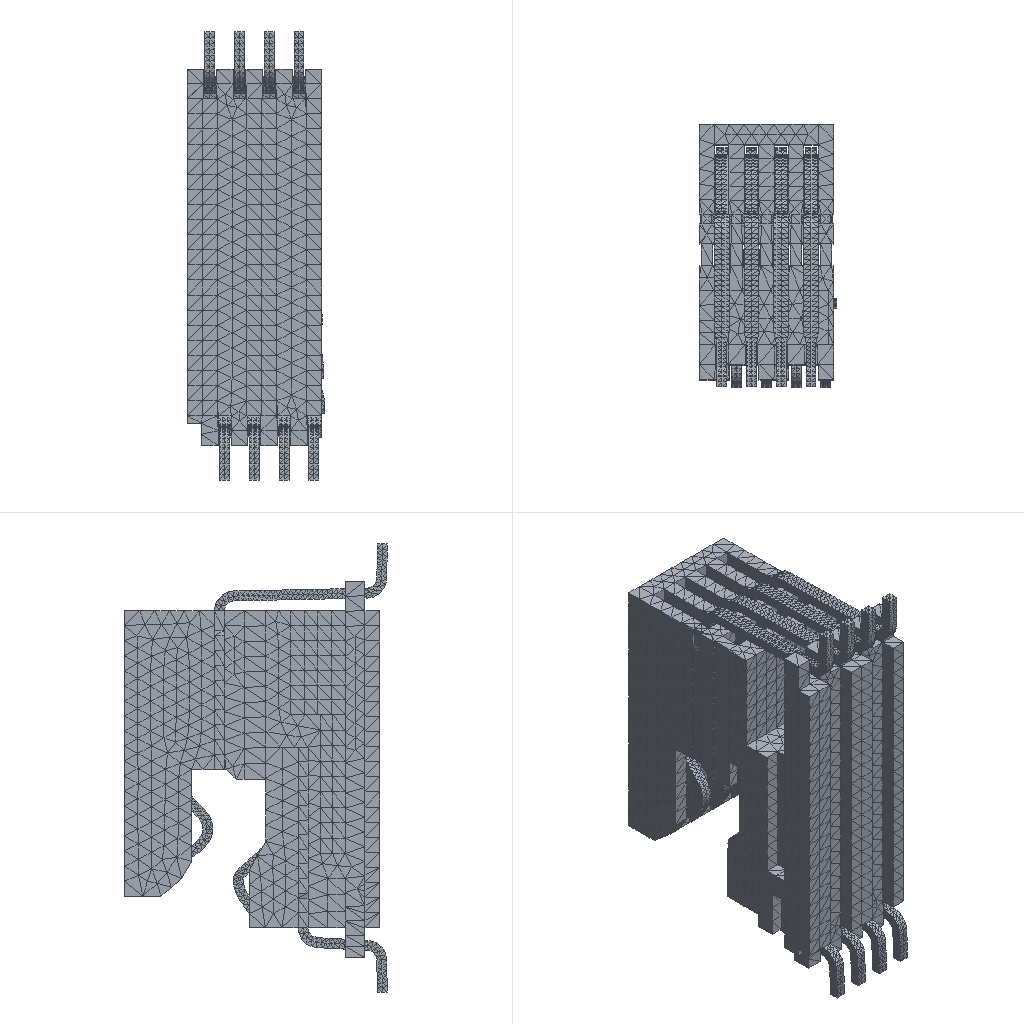Simulation study | abaqus
Set-up summary:
category,name,step,type,value,unit,region
solver,abaqus
solver,version,,,Abaqus/Standard 6.12-3
units,not stated in the deck,,not stated
analysis,deck,,coupled thermal-electrical,coupled thermal-electrical
load_step,Step-1_Temp-Ele,Step-1_Temp-Ele,coupled thermal-electrical
load_step,requested,,,1
mesh,nodes,,,107296
mesh,elements,,,59921
element_type,DC3D10E,,solid,59921
load,load commands in deck,,count,2
bc,support commands in deck,,count,2
material,C70250TM00,,in results
material,PA6T,,in results
check,setup vs results,,match,"per instance, exact: element labels, types and connectivity; labels of the nodes the elements use; coordinates of those nodes at SINGLE_PRECISION in 9 of 9 instance(s)"
Abaqus input file, long lists of numbers shortened, first 940 of 3916 lines:
*Heading
** Job name:  Model name: First_stage_TEMP-Ele
** Generated by: Abaqus/CAE 6.12-3
*Preprint, echo=NO, model=NO, history=NO, contact=NO
**
** PARTS
**
*Part, name=Housing
*Node
      1,  -9.7,  -1.59,  0.8
      2,   -7.9,  -1.59,  0.8
** (35273 more lines like these left out)
*Element, type=DC3D10E
    1,  1249,  3998,  4002,  1248,  5409,  5408,  5407,  5411,  5410,  5412
    2,  4003,  3495,   264,  1981,  5415,  5414,  5413,  5417,  5416,  5418
** (20427 more lines like these left out)
*Nset, nset=_PickedSet8, internal, generate
     1,  35275,      1
*Elset, elset=_PickedSet8, internal, generate
     1,  20429,      1
** Section: Section_PA6T
*Solid Section, elset=_PickedSet8, material=PA6T
,
*End Part
**
*Part, name=Low_T1
*Node
      1,  -7.84, -0.5128,  -1.155
      2,  -7.84,  0.2378,  -1.835
** (9275 more lines like these left out)
*Element, type=DC3D10E
   1, 1112, 1113,  412, 1114, 1521, 1520, 1519, 1523, 1522, 1524
   2, 1113, 1115, 1116, 1117, 1527, 1526, 1525, 1529, 1528, 1530
** (5131 more lines like these left out)
*Nset, nset=_PickedSet10, internal, generate
    1,  9277,     1
*Elset, elset=_PickedSet10, internal, generate
    1,  5133,     1
** Section: Section_C70250
*Solid Section, elset=_PickedSet10, material=C70250TM00
,
*End Part
**
*Part, name=Low_T2
*Node
      1,  -8.44, -0.5128,  -1.155
      2,  -8.44,  0.2378,  -1.835
** (9583 more lines like these left out)
*Element, type=DC3D10E
   1, 1123, 1124, 1125, 1126, 1561, 1560, 1559, 1563, 1562, 1564
   2, 1123, 1127, 1128, 1129, 1567, 1566, 1565, 1569, 1568, 1570
** (5348 more lines like these left out)
*Nset, nset=_PickedSet6, internal, generate
    1,  9585,     1
*Elset, elset=_PickedSet6, internal, generate
    1,  5350,     1
** Section: Section_C70250
*Solid Section, elset=_PickedSet6, material=C70250TM00
,
*End Part
**
*Part, name=Low_T3
*Node
      1,  -9.04, -0.5128,  -1.155
      2,  -9.04,  0.2378,  -1.835
** (9164 more lines like these left out)
*Element, type=DC3D10E
   1, 1113, 1114, 1115, 1116, 1509, 1508, 1507, 1511, 1510, 1512
   2, 1116, 1117,  884, 1113, 1515, 1514, 1513, 1511, 1516, 1517
** (5043 more lines like these left out)
*Nset, nset=_PickedSet8, internal, generate
    1,  9166,     1
*Elset, elset=_PickedSet8, internal, generate
    1,  5045,     1
** Section: Section_C70250
*Solid Section, elset=_PickedSet8, material=C70250TM00
,
*End Part
**
*Part, name=Low_T4
*Node
      1,  -9.64, -0.5128,  -1.155
      2,  -9.64,  0.2378,  -1.835
** (9299 more lines like these left out)
*Element, type=DC3D10E
   1, 1117, 1118, 1119, 1120, 1524, 1523, 1522, 1526, 1525, 1527
   2, 1121, 1117, 1118, 1119, 1529, 1524, 1528, 1530, 1522, 1523
** (5144 more lines like these left out)
*Nset, nset=_PickedSet6, internal, generate
    1,  9301,     1
*Elset, elset=_PickedSet6, internal, generate
    1,  5146,     1
** Section: Section_C70250
*Solid Section, elset=_PickedSet6, material=C70250TM00
,
*End Part
**
*Part, name=UP_T1
*Node
      1,  -8.15,  -2.78,   4.05
      2,  -8.15,  -2.79,         4.75
** (8647 more lines like these left out)
*Element, type=DC3D10E
   1, 1087, 1088, 1089, 1090, 1441, 1440, 1439, 1443, 1442, 1444
   2, 1087, 1091, 1092, 1093, 1447, 1446, 1445, 1449, 1448, 1450
** (4688 more lines like these left out)
*Nset, nset=_PickedSet6, internal, generate
    1,  8649,     1
*Elset, elset=_PickedSet6, internal, generate
    1,  4690,     1
** Section: Section_C70250
*Solid Section, elset=_PickedSet6, material=C70250TM00
,
*End Part
**
*Part, name=UP_T2
*Node
      1,        -8.75,  -2.78,   4.05
      2,        -8.75,  -2.79,         4.75
** (8659 more lines like these left out)
*Element, type=DC3D10E
   1, 1085, 1086, 1087,  928, 1444, 1443, 1442, 1446, 1445, 1447
   2, 1085, 1087, 1086,  893, 1442, 1443, 1444, 1449, 1448, 1450
** (4696 more lines like these left out)
*Nset, nset=_PickedSet6, internal, generate
    1,  8661,     1
*Elset, elset=_PickedSet6, internal, generate
    1,  4698,     1
** Section: Section_C70250
*Solid Section, elset=_PickedSet6, material=C70250TM00
,
*End Part
**
*Part, name=UP_T3
*Node
      1,  -9.35,  -2.78,   4.05
      2,  -9.35,  -2.79,         4.75
** (8671 more lines like these left out)
*Element, type=DC3D10E
   1, 1087,  739, 1088, 1089, 1446, 1445, 1444, 1448, 1447, 1449
   2,  555,  112, 1090, 1091, 1452, 1451, 1450, 1454, 1453, 1455
** (4702 more lines like these left out)
*Nset, nset=_PickedSet6, internal, generate
    1,  8673,     1
*Elset, elset=_PickedSet6, internal, generate
    1,  4704,     1
** Section: Section_C70250
*Solid Section, elset=_PickedSet6, material=C70250TM00
,
*End Part
**
*Part, name=UP_T4
*Node
      1,  -9.95,  -2.78,   4.05
      2,  -9.95,  -2.79,         4.75
** (8707 more lines like these left out)
*Element, type=DC3D10E
   1,  763,  747,  785, 1089, 1452, 1451, 1450, 1454, 1453, 1455
   2,  763, 1089,  657, 1090, 1454, 1457, 1456, 1459, 1458, 1460
** (4724 more lines like these left out)
*Nset, nset=_PickedSet7, internal, generate
    1,  8709,     1
*Elset, elset=_PickedSet7, internal, generate
    1,  4726,     1
** Section: Section_C70250
*Solid Section, elset=_PickedSet7, material=C70250TM00
,
*End Part
**
**
** ASSEMBLY
**
*Assembly, name=Assembly
**
*Instance, name=Housing-1, part=Housing
*End Instance
**
*Instance, name=Low_T1-1, part=Low_T1
*End Instance
**
*Instance, name=Low_T2-1, part=Low_T2
*End Instance
**
*Instance, name=Low_T3-1, part=Low_T3
*End Instance
**
*Instance, name=Low_T4-1, part=Low_T4
*End Instance
**
*Instance, name=UP_T1-1, part=UP_T1
*End Instance
**
*Instance, name=UP_T2-1, part=UP_T2
*End Instance
**
*Instance, name=UP_T3-1, part=UP_T3
*End Instance
**
*Instance, name=UP_T4-1, part=UP_T4
*End Instance
**
*Nset, nset=_PickedSet59, internal, instance=UP_T1-1
 100,
*Nset, nset=_PickedSet60, internal, instance=Low_T1-1
 5,
*Nset, nset=_PickedSet255, internal, instance=UP_T2-1
 92,
*Nset, nset=_PickedSet256, internal, instance=Low_T2-1
 5,
*Nset, nset=_PickedSet257, internal, instance=UP_T3-1
 100,
*Nset, nset=_PickedSet258, internal, instance=Low_T3-1
 5,
*Nset, nset=_PickedSet259, internal, instance=UP_T4-1
 100,
*Nset, nset=_PickedSet260, internal, instance=Low_T4-1
 5,
*Nset, nset=_PickedSet262, internal, instance=UP_T1-1
    2,    3,    5,    6,  112,  119,  120,  121,  555, 2903, 2904, 2905, 3105, 3112, 3193, 6163
 6165, 6454, 6455, 6722, 6723, 6750, 6799, 6842, 7490
*Nset, nset=_PickedSet262, internal, instance=UP_T2-1
    2,    3,    5,    6,  112,  119,  120,  121,  555, 3408, 4748, 4753, 4762, 4765, 6116, 6118
 6170, 6729, 6842, 6843, 6844, 6849, 6876, 7249, 7445
*Nset, nset=_PickedSet262, internal, instance=UP_T4-1
    2,    3,    5,    6,  112,  119,  120,  121,  555, 2951, 6387, 6389, 6391, 6675, 6678, 6687
 6688, 6750, 6779, 6874, 6918, 7030, 7342, 7559, 7560
*Nset, nset=_PickedSet262, internal, instance=UP_T3-1
    2,    3,    5,    6,  112,  119,  120,  121,  555, 1452, 2905, 2906, 2907, 5790, 5791, 5793
 6412, 6698, 6699, 6701, 6737, 6836, 6974, 7533, 7534
*Elset, elset=_PickedSet262, internal, instance=UP_T1-1
  356, 1625, 1765, 1910, 2081, 2092, 2601, 2603
*Elset, elset=_PickedSet262, internal, instance=UP_T2-1
 1661, 1679, 2026, 2091, 2101, 2378, 2609, 2611
*Elset, elset=_PickedSet262, internal, instance=UP_T4-1
 1709, 1871, 1911, 2086, 2093, 2361, 2599, 2601
*Elset, elset=_PickedSet262, internal, instance=UP_T3-1
  356, 1456, 1910, 2081, 2092, 2600, 2602, 2603
*Nset, nset=_PickedSet263, internal, instance=Low_T1-1
 33,
*Nset, nset=_PickedSet263, internal, instance=Low_T2-1
 93,
*Nset, nset=_PickedSet263, internal, instance=Low_T4-1
 33,
*Nset, nset=_PickedSet263, internal, instance=Low_T3-1
 88,
*Nset, nset=_PickedSet746, internal, instance=Housing-1, generate
     1,  35275,      1
*Nset, nset=_PickedSet746, internal, instance=Low_T1-1, generate
    1,  9277,     1
*Nset, nset=_PickedSet746, internal, instance=Low_T2-1, generate
    1,  9585,     1
*Nset, nset=_PickedSet746, internal, instance=UP_T2-1, generate
    1,  8661,     1
*Nset, nset=_PickedSet746, internal, instance=Low_T4-1, generate
    1,  9301,     1
*Nset, nset=_PickedSet746, internal, instance=UP_T4-1, generate
    1,  8709,     1
*Nset, nset=_PickedSet746, internal, instance=Low_T3-1, generate
    1,  9166,     1
*Nset, nset=_PickedSet746, internal, instance=UP_T3-1, generate
    1,  8673,     1
*Nset, nset=_PickedSet746, internal, instance=UP_T1-1, generate
    1,  8649,     1
*Elset, elset=_PickedSet746, internal, instance=Housing-1, generate
     1,  20429,      1
*Elset, elset=_PickedSet746, internal, instance=Low_T1-1, generate
    1,  5133,     1
*Elset, elset=_PickedSet746, internal, instance=Low_T2-1, generate
    1,  5350,     1
*Elset, elset=_PickedSet746, internal, instance=UP_T2-1, generate
    1,  4698,     1
*Elset, elset=_PickedSet746, internal, instance=Low_T4-1, generate
    1,  5146,     1
*Elset, elset=_PickedSet746, internal, instance=UP_T4-1, generate
    1,  4726,     1
*Elset, elset=_PickedSet746, internal, instance=Low_T3-1, generate
    1,  5045,     1
*Elset, elset=_PickedSet746, internal, instance=UP_T3-1, generate
    1,  4704,     1
*Elset, elset=_PickedSet746, internal, instance=UP_T1-1, generate
    1,  4690,     1
*Nset, nset=_PickedSet1712, internal, instance=Low_T1-1
   33,   34,   35,   36,  263,  265,  266,  267,  268,  269,  270,  271,  272,  273,  274,  275
  660,  661,  662,  663,  664, 3312, 3320, 4258, 4280, 4541, 4880, 4883, 4884, 5596, 7014, 7428
** (3 more lines like these left out)
*Nset, nset=_PickedSet1712, internal, instance=Low_T2-1
   93,   94,   95,   96,  449,  451,  452,  453,  454,  455,  456,  457,  458,  459,  460,  461
  978,  979,  980,  981,  982, 1848, 3815, 5830, 5832, 5833, 5924, 6047, 6048, 6068, 6069, 6071
** (3 more lines like these left out)
*Nset, nset=_PickedSet1712, internal, instance=Low_T4-1
   33,   34,   35,   36,  266,  268,  269,  270,  271,  272,  273,  274,  275,  276,  277,  278
  663,  664,  665,  666,  667, 4509, 5722, 5727, 5729, 5939, 6122, 6702, 6704, 6705, 6706, 6763
** (3 more lines like these left out)
*Nset, nset=_PickedSet1712, internal, instance=UP_T2-1
    1,    2,    3,    4,  107,  108,  109,  110,  111,  112,  113,  114,  115,  116,  117,  118
  550,  551,  552,  553,  554, 3413, 3422, 3580, 3581, 3598, 3613, 6109, 6150, 6172, 6206, 6207
** (3 more lines like these left out)
*Nset, nset=_PickedSet1712, internal, instance=UP_T4-1
    1,    2,    3,    4,  107,  108,  109,  110,  111,  112,  113,  114,  115,  116,  117,  118
  550,  551,  552,  553,  554, 4174, 4206, 4208, 4209, 5555, 5558, 6265, 6267, 6276, 6531, 6532
** (3 more lines like these left out)
*Nset, nset=_PickedSet1712, internal, instance=Low_T3-1
   83,   84,   87,   88,  424,  436,  437,  438,  439,  440,  441,  442,  443,  444,  445,  446
  969,  970,  971,  972,  973, 4906, 4907, 4908, 5571, 5573, 5574, 5585, 5662, 6557, 6559, 6560
** (3 more lines like these left out)
*Nset, nset=_PickedSet1712, internal, instance=UP_T3-1
    1,    2,    3,    4,  107,  108,  109,  110,  111,  112,  113,  114,  115,  116,  117,  118
  550,  551,  552,  553,  554, 3667, 3668, 3693, 3702, 3703, 6172, 6181, 6409, 6412, 6413, 6468
** (3 more lines like these left out)
*Nset, nset=_PickedSet1712, internal, instance=UP_T1-1
    1,    2,    3,    4,  107,  108,  109,  110,  111,  112,  113,  114,  115,  116,  117,  118
  550,  551,  552,  553,  554, 3078, 3096, 3196, 3205, 6162, 6196, 6200, 6201, 6207, 6455, 6456
** (3 more lines like these left out)
*Elset, elset=_PickedSet1712, internal, instance=Low_T1-1
  997, 3072, 3074, 3189, 3372, 3450, 3726, 3746, 3768, 3795, 3802, 3819, 3823, 3829, 3834, 3843
 3857, 3868, 3881, 3895, 3904, 3908, 5119, 5132
*Elset, elset=_PickedSet1712, internal, instance=Low_T2-1
 1362, 1463, 1470, 1473, 1730, 1832, 3902, 3914, 3916, 4409, 4416, 4417, 4545, 4553, 4569, 4576
 4596, 4602, 4620, 4635, 4636, 4666, 4684, 4711
*Elset, elset=_PickedSet1712, internal, instance=Low_T4-1
 1783, 1808, 3633, 3651, 3669, 3699, 3742, 3743, 3745, 3761, 3788, 3820, 3821, 3832, 3833, 3842
 3852, 3859, 3888, 3893, 4823, 4926, 5086, 5140
*Elset, elset=_PickedSet1712, internal, instance=UP_T2-1
 1654, 1672, 1700, 1795, 1901, 1907, 1916, 1925, 1938, 1940, 1941, 1947, 1955, 1960, 1977, 1984
 2003, 2024, 2068, 2070, 2081, 2350, 2379, 2587
*Elset, elset=_PickedSet1712, internal, instance=UP_T4-1
  736, 1289, 1649, 1788, 1886, 1892, 1901, 1910, 1923, 1926, 1931, 1938, 1942, 1950, 1959, 1969
 1984, 2049, 2054, 2065, 2137, 2333, 2361, 2577
*Elset, elset=_PickedSet1712, internal, instance=Low_T3-1
 1004, 1258, 1723, 1749, 1858, 2126, 3380, 3575, 4203, 4231, 4253, 4266, 4268, 4278, 4292, 4294
 4297, 4304, 4306, 4308, 4311, 4312, 4319, 4321
*Elset, elset=_PickedSet1712, internal, instance=UP_T3-1
  580, 1649, 1765, 1789, 1891, 1901, 1905, 1909, 1922, 1925, 1930, 1937, 1941, 1949, 1958, 1968
 1983, 2006, 2048, 2053, 2063, 2112, 2332, 2578
*Elset, elset=_PickedSet1712, internal, instance=UP_T1-1
 1649, 1765, 1789, 1885, 1891, 1900, 1909, 1922, 1924, 1925, 1930, 1937, 1941, 1949, 1958, 1968
 1983, 2006, 2019, 2048, 2053, 2063, 2333, 2579
*Elset, elset=_CP-1-Housing-1_S3, internal, instance=Housing-1
   406,   432,  3378,  3381,  4906,  4937,  5048,  5058,  5204,  5520,  5575,  5749,  5980,  6251,  6610,  6617
  6630,  6658,  6678,  6756,  6990,  7061,  7074,  7080,  7093,  7105,  7117,  7148,  7407,  7460,  7519,  7536
** (10 more lines like these left out)
*Elset, elset=_CP-1-Housing-1_S2, internal, instance=Housing-1
  1197,  6526,  8877,  9151,  9215, 14120
*Elset, elset=_CP-1-Housing-1_S4, internal, instance=Housing-1
 2427, 4753, 6544, 9248
*Elset, elset=_CP-1-Housing-1_S1, internal, instance=Housing-1
 5201,
*Surface, type=ELEMENT, name=CP-1-Housing-1
_CP-1-Housing-1_S3, S3
_CP-1-Housing-1_S2, S2
_CP-1-Housing-1_S4, S4
_CP-1-Housing-1_S1, S1
*Elset, elset=_CP-1-Low_T1-1_S3, internal, instance=Low_T1-1
 1954, 2376, 3715, 5002
*Surface, type=ELEMENT, name=CP-1-Low_T1-1
_CP-1-Low_T1-1_S3, S3
*Elset, elset=_CP-2-Housing-1_S3, internal, instance=Housing-1
 2269, 5226, 9646, 9648
*Surface, type=ELEMENT, name=CP-2-Housing-1
_CP-2-Housing-1_S3, S3
*Elset, elset=_CP-2-Low_T1-1_S1, internal, instance=Low_T1-1
 1936,
*Elset, elset=_CP-2-Low_T1-1_S4, internal, instance=Low_T1-1
 2193, 3856
*Elset, elset=_CP-2-Low_T1-1_S3, internal, instance=Low_T1-1
 3757,
*Surface, type=ELEMENT, name=CP-2-Low_T1-1
_CP-2-Low_T1-1_S1, S1
_CP-2-Low_T1-1_S4, S4
_CP-2-Low_T1-1_S3, S3
*Elset, elset=_CP-3-Housing-1_S3, internal, instance=Housing-1
 2269, 5226, 9646, 9648
*Surface, type=ELEMENT, name=CP-3-Housing-1
_CP-3-Housing-1_S3, S3
*Elset, elset=_CP-3-Low_T1-1_S3, internal, instance=Low_T1-1
 2278, 3658, 3847, 3850
*Surface, type=ELEMENT, name=CP-3-Low_T1-1
_CP-3-Low_T1-1_S3, S3
*Elset, elset=_CP-4-Housing-1_S4, internal, instance=Housing-1
 1431, 6407, 8578, 9690, 9716, 9751
*Elset, elset=_CP-4-Housing-1_S1, internal, instance=Housing-1
 4838,
*Elset, elset=_CP-4-Housing-1_S3, internal, instance=Housing-1
  5955,  6485,  6501,  8375,  8462,  9457,  9707,  9724,  9726,  9734,  9743,  9744,  9782,  9856, 11574, 11601
 11851,
*Elset, elset=_CP-4-Housing-1_S2, internal, instance=Housing-1
 11676,
*Surface, type=ELEMENT, name=CP-4-Housing-1
_CP-4-Housing-1_S4, S4
_CP-4-Housing-1_S1, S1
_CP-4-Housing-1_S2, S2
_CP-4-Housing-1_S3, S3
*Elset, elset=_CP-4-Low_T1-1_S3, internal, instance=Low_T1-1
  131,  200,  205,  220,  256,  280,  296,  303,  307,  309,  311,  345,  357,  415,  460,  490
  522,  560,  590,  618,  653,  668,  671,  685,  690,  696,  759,  767,  769,  771,  772,  776
** (28 more lines like these left out)
*Elset, elset=_CP-4-Low_T1-1_S1, internal, instance=Low_T1-1
   12,  208,  377,  495,  971, 1006, 1191, 1374, 1377, 1414, 1829, 2029, 2193, 2293, 2391, 2425
 2605, 2793, 2826, 3046, 3188, 3336, 3366, 3428, 3449, 3457, 3477, 3485, 3500, 4070, 4089, 4200
** (1 more lines like these left out)
*Elset, elset=_CP-4-Low_T1-1_S4, internal, instance=Low_T1-1
  113,  166,  210,  355,  478,  545,  610,  894, 1081, 1289, 1309, 1378, 1493, 1505, 1573, 1613
 1632, 1683, 1775, 1867, 2031, 2077, 2118, 2135, 2252, 2254, 2344, 2572, 2640, 2794, 2877, 3076
** (3 more lines like these left out)
*Elset, elset=_CP-4-Low_T1-1_S2, internal, instance=Low_T1-1
 1419, 1756, 1759, 1768, 2132, 2138, 2296, 2374, 2418, 2440, 2451, 2467, 2588, 2627, 2654, 2666
 2801, 2831, 2870, 3041, 3190, 3213, 3276, 3357, 3385, 3389, 3447, 3695, 3870, 3901, 3935, 3937
** (2 more lines like these left out)
*Surface, type=ELEMENT, name=CP-4-Low_T1-1
_CP-4-Low_T1-1_S3, S3
_CP-4-Low_T1-1_S1, S1
_CP-4-Low_T1-1_S4, S4
_CP-4-Low_T1-1_S2, S2
*Elset, elset=_CP-5-Housing-1_S3, internal, instance=Housing-1
  3760,  4126,  5421,  5619,  5792,  5931,  6406,  6418,  6425,  6456,  6467,  6476,  6483,  6495,  6500,  8390
  9687,  9887, 10636, 11571, 11747, 11814, 11850, 11930, 12367, 12928
*Surface, type=ELEMENT, name=CP-5-Housing-1
_CP-5-Housing-1_S3, S3
*Elset, elset=_CP-5-Low_T1-1_S3, internal, instance=Low_T1-1
  423,  684,  849, 1203, 1289, 1394, 2261, 2374, 2428, 2587, 4132, 4145, 4150, 4167, 4170, 4176
 4212, 4238, 4262, 4272, 4294, 4296, 4513
*Elset, elset=_CP-5-Low_T1-1_S4, internal, instance=Low_T1-1
  621, 1420, 1836, 4286, 4326, 4775
*Elset, elset=_CP-5-Low_T1-1_S2, internal, instance=Low_T1-1
 2053, 4043
*Elset, elset=_CP-5-Low_T1-1_S1, internal, instance=Low_T1-1
 4143,
*Surface, type=ELEMENT, name=CP-5-Low_T1-1
_CP-5-Low_T1-1_S3, S3
_CP-5-Low_T1-1_S4, S4
_CP-5-Low_T1-1_S2, S2
_CP-5-Low_T1-1_S1, S1
*Elset, elset=_CP-6-Housing-1_S4, internal, instance=Housing-1
   544, 13221
*Elset, elset=_CP-6-Housing-1_S3, internal, instance=Housing-1
  5936,  6411,  6438,  6464,  8446,  8689,  9669,  9689,  9721, 13227, 13253, 13255, 13256, 13257, 13259, 13313
 14533, 14537, 16066, 16087, 16088, 16128, 16168, 16205
*Surface, type=ELEMENT, name=CP-6-Housing-1
_CP-6-Housing-1_S4, S4
_CP-6-Housing-1_S3, S3
*Elset, elset=_CP-6-Low_T1-1_S4, internal, instance=Low_T1-1
   27,  147,  997, 1195, 1196, 1207, 1317, 1471, 1648, 1679, 1686, 1715, 1722, 1785, 1817, 1870
 1904, 1907, 2047, 2266, 2379, 2507, 2568, 2596, 2726, 2761, 2769, 2822, 3062, 3114, 3204, 3234
** (2 more lines like these left out)
*Elset, elset=_CP-6-Low_T1-1_S3, internal, instance=Low_T1-1
   66,  130,  146,  191,  218,  240,  265,  285,  351,  372,  379,  409,  431,  487,  533,  563
  601,  605,  609,  665,  730,  792,  808,  818,  834,  839,  851,  915,  922,  924,  975, 1014
** (30 more lines like these left out)
*Elset, elset=_CP-6-Low_T1-1_S2, internal, instance=Low_T1-1
  190,  261,  651,  837,  921,  925, 1011, 1206, 1220, 1321, 1436, 1501, 1984, 2016, 2146, 2156
 2746, 2803, 2860, 2885, 2918, 3059, 3082, 3104, 3119, 3178, 3387, 3502, 3518, 3532, 3545, 3641
** (2 more lines like these left out)
*Elset, elset=_CP-6-Low_T1-1_S1, internal, instance=Low_T1-1
  397,  419,  539,  684,  731, 1209, 1284, 1415, 1449, 1503, 1631, 2256, 2304, 2476, 2488, 2540
 2649, 2778, 3024, 3081, 3146, 3200, 3527, 3529, 3549, 3703, 3819, 3843, 3856, 4099, 4116, 4161
** (1 more lines like these left out)
*Surface, type=ELEMENT, name=CP-6-Low_T1-1
_CP-6-Low_T1-1_S4, S4
_CP-6-Low_T1-1_S3, S3
_CP-6-Low_T1-1_S2, S2
_CP-6-Low_T1-1_S1, S1
*Elset, elset=_CP-7-Housing-1_S3, internal, instance=Housing-1
  3760,  4126,  5421,  5619,  5792,  5931,  6406,  6418,  6425,  6456,  6467,  6476,  6483,  6495,  6500,  8390
  9687,  9887, 10636, 11571, 11747, 11814, 11850, 11930, 12367, 12928
*Surface, type=ELEMENT, name=CP-7-Housing-1
_CP-7-Housing-1_S3, S3
*Elset, elset=_CP-7-Low_T1-1_S4, internal, instance=Low_T1-1
  261,  539, 1010, 1011, 1121, 1229, 1375, 1504, 1759, 1937, 2016, 2022, 2074, 2106, 2116, 2146
 2201, 2304, 2339, 2481, 2605, 2657, 2666, 2749, 2803, 2827, 2831, 2838, 2913, 2918, 2983, 2991
** (2 more lines like these left out)
*Elset, elset=_CP-7-Low_T1-1_S3, internal, instance=Low_T1-1
  214,  297,  413,  495,  536,  542,  551,  631,  675,  728,  741,  742,  862,  905,  943,  950
  952,  999, 1007, 1022, 1045, 1067, 1069, 1070, 1123, 1126, 1129, 1210, 1211, 1238, 1241, 1344
** (10 more lines like these left out)
*Elset, elset=_CP-7-Low_T1-1_S1, internal, instance=Low_T1-1
  629, 1093, 1680, 1974, 2132, 2135, 2268, 2354, 2553, 2571, 2946, 2955, 2992, 3921, 4320, 4639
 4687, 4702
*Elset, elset=_CP-7-Low_T1-1_S2, internal, instance=Low_T1-1
    3, 1195, 1207, 1240, 1672, 1720, 1944, 1968, 1993, 2098, 2199, 2608, 2655, 2725, 2822, 2849
 2963, 3036, 3044, 3066, 3111, 3561, 3960, 3963, 3990, 4659, 4905, 4940, 4942, 4975, 5029
*Surface, type=ELEMENT, name=CP-7-Low_T1-1
_CP-7-Low_T1-1_S4, S4
_CP-7-Low_T1-1_S3, S3
_CP-7-Low_T1-1_S2, S2
_CP-7-Low_T1-1_S1, S1
*Elset, elset=_CP-8-Housing-1_S3, internal, instance=Housing-1
   654,  1431,  2563,  2567,  3448,  5209,  5417,  6127,  6942,  6949,  8482,  9446,  9758,  9779,  9783,  9854
  9873,  9990, 11331, 11556, 11558, 11570, 11575, 11595, 11597, 11603, 11606, 11635, 11643, 11647, 11669, 11712
** (1 more lines like these left out)
*Elset, elset=_CP-8-Housing-1_S4, internal, instance=Housing-1
  4838,  5908, 11676, 11864
*Elset, elset=_CP-8-Housing-1_S2, internal, instance=Housing-1
  5661,  6407,  8462,  8578,  9707,  9716, 11591, 11879
*Elset, elset=_CP-8-Housing-1_S1, internal, instance=Housing-1
  9726,  9744,  9751, 11561, 11574, 11648, 11703
*Surface, type=ELEMENT, name=CP-8-Housing-1
_CP-8-Housing-1_S3, S3
_CP-8-Housing-1_S4, S4
_CP-8-Housing-1_S2, S2
_CP-8-Housing-1_S1, S1
*Elset, elset=_CP-8-Low_T1-1_S4, internal, instance=Low_T1-1
  261,  539, 1010, 1011, 1121, 1229, 1375, 1504, 1759, 1937, 2016, 2022, 2074, 2106, 2116, 2146
 2201, 2304, 2339, 2481, 2605, 2657, 2666, 2749, 2803, 2827, 2831, 2838, 2913, 2918, 2983, 2991
** (2 more lines like these left out)
*Elset, elset=_CP-8-Low_T1-1_S3, internal, instance=Low_T1-1
  214,  297,  413,  495,  536,  542,  551,  631,  675,  728,  741,  742,  862,  905,  943,  950
  952,  999, 1007, 1022, 1045, 1067, 1069, 1070, 1123, 1126, 1129, 1210, 1211, 1238, 1241, 1344
** (10 more lines like these left out)
*Elset, elset=_CP-8-Low_T1-1_S1, internal, instance=Low_T1-1
  629, 1093, 1680, 1974, 2132, 2135, 2268, 2354, 2553, 2571, 2946, 2955, 2992, 3921, 4320, 4639
 4687, 4702
*Elset, elset=_CP-8-Low_T1-1_S2, internal, instance=Low_T1-1
    3, 1195, 1207, 1240, 1672, 1720, 1944, 1968, 1993, 2098, 2199, 2608, 2655, 2725, 2822, 2849
 2963, 3036, 3044, 3066, 3111, 3561, 3960, 3963, 3990, 4659, 4905, 4940, 4942, 4975, 5029
*Surface, type=ELEMENT, name=CP-8-Low_T1-1
_CP-8-Low_T1-1_S4, S4
_CP-8-Low_T1-1_S3, S3
_CP-8-Low_T1-1_S2, S2
_CP-8-Low_T1-1_S1, S1
*Elset, elset=_CP-9-Housing-1_S3, internal, instance=Housing-1
   406,   432,  3378,  3381,  4906,  4937,  5048,  5058,  5204,  5520,  5575,  5749,  5980,  6251,  6610,  6617
  6630,  6658,  6678,  6756,  6990,  7061,  7074,  7080,  7093,  7105,  7117,  7148,  7407,  7460,  7519,  7536
** (10 more lines like these left out)
*Elset, elset=_CP-9-Housing-1_S2, internal, instance=Housing-1
  1197,  6526,  8877,  9151,  9215, 14120
*Elset, elset=_CP-9-Housing-1_S4, internal, instance=Housing-1
 2427, 4753, 6544, 9248
*Elset, elset=_CP-9-Housing-1_S1, internal, instance=Housing-1
 5201,
*Surface, type=ELEMENT, name=CP-9-Housing-1
_CP-9-Housing-1_S3, S3
_CP-9-Housing-1_S2, S2
_CP-9-Housing-1_S4, S4
_CP-9-Housing-1_S1, S1
*Elset, elset=_CP-9-Low_T2-1_S3, internal, instance=Low_T2-1
 1059, 1267, 4152, 4160
*Surface, type=ELEMENT, name=CP-9-Low_T2-1
_CP-9-Low_T2-1_S3, S3
*Elset, elset=_CP-10-Housing-1_S3, internal, instance=Housing-1
   406,   432,  3378,  3381,  4906,  4937,  5048,  5058,  5204,  5520,  5575,  5749,  5980,  6251,  6610,  6617
  6630,  6658,  6678,  6756,  6990,  7061,  7074,  7080,  7093,  7105,  7117,  7148,  7407,  7460,  7519,  7536
** (10 more lines like these left out)
*Elset, elset=_CP-10-Housing-1_S2, internal, instance=Housing-1
  1197,  6526,  8877,  9151,  9215, 14120
*Elset, elset=_CP-10-Housing-1_S4, internal, instance=Housing-1
 2427, 4753, 6544, 9248
*Elset, elset=_CP-10-Housing-1_S1, internal, instance=Housing-1
 5201,
*Surface, type=ELEMENT, name=CP-10-Housing-1
_CP-10-Housing-1_S3, S3
_CP-10-Housing-1_S2, S2
_CP-10-Housing-1_S4, S4
_CP-10-Housing-1_S1, S1
*Elset, elset=_CP-10-Low_T2-1_S3, internal, instance=Low_T2-1
 2848, 2850
*Elset, elset=_CP-10-Low_T2-1_S2, internal, instance=Low_T2-1
 4370, 4693
*Surface, type=ELEMENT, name=CP-10-Low_T2-1
_CP-10-Low_T2-1_S3, S3
_CP-10-Low_T2-1_S2, S2
*Elset, elset=_CP-11-Housing-1_S3, internal, instance=Housing-1
 5668, 6584, 6586, 7261
*Surface, type=ELEMENT, name=CP-11-Housing-1
_CP-11-Housing-1_S3, S3
*Elset, elset=_CP-11-Low_T2-1_S3, internal, instance=Low_T2-1
 4368, 4371, 4467, 4700
*Surface, type=ELEMENT, name=CP-11-Low_T2-1
_CP-11-Low_T2-1_S3, S3
*Elset, elset=_CP-12-Housing-1_S3, internal, instance=Housing-1
 5668, 6584, 6586, 7261
*Surface, type=ELEMENT, name=CP-12-Housing-1
_CP-12-Housing-1_S3, S3
*Elset, elset=_CP-12-Low_T2-1_S3, internal, instance=Low_T2-1
 4384, 4385, 4387, 4389
*Surface, type=ELEMENT, name=CP-12-Low_T2-1
_CP-12-Low_T2-1_S3, S3
*Elset, elset=_CP-13-Housing-1_S3, internal, instance=Housing-1
 5180, 6558, 8994
*Elset, elset=_CP-13-Housing-1_S4, internal, instance=Housing-1
 5221,
*Surface, type=ELEMENT, name=CP-13-Housing-1
_CP-13-Housing-1_S3, S3
_CP-13-Housing-1_S4, S4
*Elset, elset=_CP-13-Low_T2-1_S4, internal, instance=Low_T2-1
 3591, 3974
*Elset, elset=_CP-13-Low_T2-1_S3, internal, instance=Low_T2-1
 4027, 4034
*Surface, type=ELEMENT, name=CP-13-Low_T2-1
_CP-13-Low_T2-1_S4, S4
_CP-13-Low_T2-1_S3, S3
*Elset, elset=_CP-14-Housing-1_S3, internal, instance=Housing-1
 5180, 6558, 8994
*Elset, elset=_CP-14-Housing-1_S4, internal, instance=Housing-1
 5221,
*Surface, type=ELEMENT, name=CP-14-Housing-1
_CP-14-Housing-1_S3, S3
_CP-14-Housing-1_S4, S4
*Elset, elset=_CP-14-Low_T2-1_S3, internal, instance=Low_T2-1
  842,  985, 1885, 3875
*Surface, type=ELEMENT, name=CP-14-Low_T2-1
_CP-14-Low_T2-1_S3, S3
*Elset, elset=_CP-15-Housing-1_S4, internal, instance=Housing-1
  2670,  5554,  5870, 10058, 12097
*Elset, elset=_CP-15-Housing-1_S3, internal, instance=Housing-1
  4331,  5036,  5120,  5220,  5787,  5934,  9789,  9872,  9936, 11739, 11995, 12266, 14560
*Elset, elset=_CP-15-Housing-1_S1, internal, instance=Housing-1
  5884,  6167, 11629, 11841
*Elset, elset=_CP-15-Housing-1_S2, internal, instance=Housing-1
  5922, 11881, 11938
*Surface, type=ELEMENT, name=CP-15-Housing-1
_CP-15-Housing-1_S4, S4
_CP-15-Housing-1_S3, S3
_CP-15-Housing-1_S2, S2
_CP-15-Housing-1_S1, S1
*Elset, elset=_CP-15-Low_T2-1_S3, internal, instance=Low_T2-1
   67,  225,  278,  315,  324,  351,  356,  361,  373,  381,  397,  399,  413,  418,  468,  495
  518,  528,  557,  586,  628,  656,  657,  708,  725,  732,  761,  769,  791,  794,  796,  813
** (30 more lines like these left out)
*Elset, elset=_CP-15-Low_T2-1_S1, internal, instance=Low_T2-1
  248,  606,  786, 1049, 1448, 1934, 2051, 2054, 2056, 2169, 2271, 2332, 2340, 2360, 2372, 2395
 2405, 2493, 2514, 2681, 2886, 2889, 2927, 2981, 3038, 3186, 3256, 3295, 3323, 3625, 3732, 3946
** (1 more lines like these left out)
*Elset, elset=_CP-15-Low_T2-1_S4, internal, instance=Low_T2-1
   28,  474,  554,  603,  755,  883,  987, 1029, 1121, 1281, 1287, 1571, 1588, 1612, 1659, 1715
 1821, 1838, 1871, 1900, 1973, 2039, 2139, 2157, 2336, 2406, 2412, 2430, 2501, 2547, 2827, 2868
** (2 more lines like these left out)
*Elset, elset=_CP-15-Low_T2-1_S2, internal, instance=Low_T2-1
  334,  610, 1056, 1161, 1211, 1589, 1779, 2250, 2686, 2695, 2814, 2878, 2996, 3230, 3344, 3611
 3623, 3719, 3736, 3962, 3978, 3981, 4121, 4137, 4179, 4217, 4256, 4293, 4310, 4337, 4343, 4450
** (1 more lines like these left out)
*Surface, type=ELEMENT, name=CP-15-Low_T2-1
_CP-15-Low_T2-1_S3, S3
_CP-15-Low_T2-1_S1, S1
_CP-15-Low_T2-1_S4, S4
_CP-15-Low_T2-1_S2, S2
*Elset, elset=_CP-16-Housing-1_S4, internal, instance=Housing-1
  3928,  5174,  9828, 11971
*Elset, elset=_CP-16-Housing-1_S1, internal, instance=Housing-1
  5605,  9998, 10000, 11717, 11788
*Elset, elset=_CP-16-Housing-1_S3, internal, instance=Housing-1
  5932,  6408,  6440,  8499,  9865,  9890,  9892,  9898,  9899,  9903,  9904,  9951, 10008, 12234
*Elset, elset=_CP-16-Housing-1_S2, internal, instance=Housing-1
  9768, 10012
*Surface, type=ELEMENT, name=CP-16-Housing-1
_CP-16-Housing-1_S4, S4
_CP-16-Housing-1_S1, S1
_CP-16-Housing-1_S2, S2
_CP-16-Housing-1_S3, S3
*Elset, elset=_CP-16-Low_T2-1_S3, internal, instance=Low_T2-1
   67,  225,  278,  315,  324,  351,  356,  361,  373,  381,  397,  399,  413,  418,  468,  495
  518,  528,  557,  586,  628,  656,  657,  708,  725,  732,  761,  769,  791,  794,  796,  813
** (30 more lines like these left out)
*Elset, elset=_CP-16-Low_T2-1_S1, internal, instance=Low_T2-1
  248,  606,  786, 1049, 1448, 1934, 2051, 2054, 2056, 2169, 2271, 2332, 2340, 2360, 2372, 2395
 2405, 2493, 2514, 2681, 2886, 2889, 2927, 2981, 3038, 3186, 3256, 3295, 3323, 3625, 3732, 3946
** (1 more lines like these left out)
*Elset, elset=_CP-16-Low_T2-1_S4, internal, instance=Low_T2-1
   28,  474,  554,  603,  755,  883,  987, 1029, 1121, 1281, 1287, 1571, 1588, 1612, 1659, 1715
 1821, 1838, 1871, 1900, 1973, 2039, 2139, 2157, 2336, 2406, 2412, 2430, 2501, 2547, 2827, 2868
** (2 more lines like these left out)
*Elset, elset=_CP-16-Low_T2-1_S2, internal, instance=Low_T2-1
  334,  610, 1056, 1161, 1211, 1589, 1779, 2250, 2686, 2695, 2814, 2878, 2996, 3230, 3344, 3611
 3623, 3719, 3736, 3962, 3978, 3981, 4121, 4137, 4179, 4217, 4256, 4293, 4310, 4337, 4343, 4450
** (1 more lines like these left out)
*Surface, type=ELEMENT, name=CP-16-Low_T2-1
_CP-16-Low_T2-1_S3, S3
_CP-16-Low_T2-1_S1, S1
_CP-16-Low_T2-1_S4, S4
_CP-16-Low_T2-1_S2, S2
*Elset, elset=_CP-17-Housing-1_S3, internal, instance=Housing-1
  1539,  3700,  4128,  4800,  5604,  5641,  5848,  5866,  5873,  5893,  5946,  5951,  6384,  6430,  6434,  6463
  7152,  7242,  9821,  9832,  9858,  9953, 10260, 10629, 11946, 12925
*Surface, type=ELEMENT, name=CP-17-Housing-1
_CP-17-Housing-1_S3, S3
*Elset, elset=_CP-17-Low_T2-1_S4, internal, instance=Low_T2-1
  903, 4887, 5069, 5115, 5131, 5263
*Elset, elset=_CP-17-Low_T2-1_S3, internal, instance=Low_T2-1
  721,  994, 1212, 2302, 2372, 3762, 3780, 3871, 4847, 4874, 5097, 5212, 5282, 5289, 5299, 5302
 5317, 5327, 5332, 5338, 5341, 5345
*Elset, elset=_CP-17-Low_T2-1_S2, internal, instance=Low_T2-1
 3895,
*Elset, elset=_CP-17-Low_T2-1_S1, internal, instance=Low_T2-1
 1606, 3796, 5342
*Surface, type=ELEMENT, name=CP-17-Low_T2-1
_CP-17-Low_T2-1_S4, S4
_CP-17-Low_T2-1_S3, S3
_CP-17-Low_T2-1_S2, S2
_CP-17-Low_T2-1_S1, S1
*Elset, elset=_CP-18-Housing-1_S3, internal, instance=Housing-1
  4867,  5740,  5754,  5757,  5776,  5786,  5790,  5810,  5811,  5889,  5992,  6056,  6111,  6114,  6130,  6150
  6890,  8912,  9879,  9880,  9962,  9966,  9975, 18337
*Elset, elset=_CP-18-Housing-1_S2, internal, instance=Housing-1
 5603, 5657
*Surface, type=ELEMENT, name=CP-18-Housing-1
_CP-18-Housing-1_S3, S3
_CP-18-Housing-1_S2, S2
*Elset, elset=_CP-18-Low_T2-1_S3, internal, instance=Low_T2-1
  562, 1779, 1862, 2236, 2343, 2403, 3773, 3784, 3793, 3799, 3804, 3847, 3865, 3879, 3893, 5046
 5220, 5243, 5244, 5247, 5270, 5283, 5312, 5324
*Elset, elset=_CP-18-Low_T2-1_S1, internal, instance=Low_T2-1
  787, 3016, 3820, 3860
*Elset, elset=_CP-18-Low_T2-1_S4, internal, instance=Low_T2-1
 2250, 2893, 5087
*Elset, elset=_CP-18-Low_T2-1_S2, internal, instance=Low_T2-1
 3903,
*Surface, type=ELEMENT, name=CP-18-Low_T2-1
_CP-18-Low_T2-1_S3, S3
_CP-18-Low_T2-1_S1, S1
_CP-18-Low_T2-1_S4, S4
_CP-18-Low_T2-1_S2, S2
*Elset, elset=_CP-19-Housing-1_S3, internal, instance=Housing-1
  5549,  5568,  5636,  5733,  5818,  5827,  5852,  5859,  5900,  5913,  5930,  6623,  7087,  7094,  7095,  8454
  8455,  8465,  8469,  8479,  8568,  8611,  8618,  9829,  9930,  9937,  9950, 10358, 10363, 14513
*Elset, elset=_CP-19-Housing-1_S2, internal, instance=Housing-1
 5735, 9929
*Surface, type=ELEMENT, name=CP-19-Housing-1
_CP-19-Housing-1_S3, S3
_CP-19-Housing-1_S2, S2
*Elset, elset=_CP-19-Low_T2-1_S2, internal, instance=Low_T2-1
  343, 1269, 1319, 1750, 1964, 2176, 2198, 2262, 2635, 2642, 2863, 2900, 2914, 3018, 3042, 3084
 3091, 3122, 3189, 3200, 3397, 3478, 3622, 3800, 3860, 3880, 4076, 4084, 4107, 4129, 4161, 4166
** (1 more lines like these left out)
*Elset, elset=_CP-19-Low_T2-1_S3, internal, instance=Low_T2-1
   22,   36,   38,   71,  117,  120,  163,  183,  249,  262,  291,  375,  444,  545,  565,  640
  643,  700,  734,  775,  806,  820,  879,  882,  894,  901,  904,  908,  934,  967, 1040, 1044
** (30 more lines like these left out)
*Elset, elset=_CP-19-Low_T2-1_S1, internal, instance=Low_T2-1
  194,  721,  731, 1276, 1388, 1503, 1913, 1929, 1950, 1970, 2166, 2203, 2417, 3074, 3325, 3409
 3461, 3482, 3746, 3930, 3975, 4205, 4218, 4249, 4324, 4366, 4416, 4545, 4547, 4666, 4684, 4765
** (1 more lines like these left out)
*Elset, elset=_CP-19-Low_T2-1_S4, internal, instance=Low_T2-1
   45,  167,  519,  568,  833,  896,  906, 1081, 1261, 1362, 1406, 1463, 1535, 1670, 1735, 1799
 1939, 2160, 2321, 2730, 2759, 2817, 2922, 2960, 2999, 3165, 3396, 3449, 3501, 3510, 3515, 3521
** (3 more lines like these left out)
*Surface, type=ELEMENT, name=CP-19-Low_T2-1
_CP-19-Low_T2-1_S2, S2
_CP-19-Low_T2-1_S3, S3
_CP-19-Low_T2-1_S4, S4
_CP-19-Low_T2-1_S1, S1
*Elset, elset=_CP-20-Housing-1_S3, internal, instance=Housing-1
  1539,  3700,  4128,  4800,  5604,  5641,  5848,  5866,  5873,  5893,  5946,  5951,  6384,  6430,  6434,  6463
  7152,  7242,  9821,  9832,  9858,  9953, 10260, 10629, 11946, 12925
*Surface, type=ELEMENT, name=CP-20-Housing-1
_CP-20-Housing-1_S3, S3
*Elset, elset=_CP-20-Low_T2-1_S3, internal, instance=Low_T2-1
  445,  515,  575,  581,  584,  585,  680,  681,  684,  693,  695,  741,  776,  812, 1035, 1036
 1039, 1100, 1243, 1245, 1306, 1307, 1378, 1391, 1392, 1494, 1496, 1499, 1513, 1703, 1719, 1726
** (11 more lines like these left out)
*Elset, elset=_CP-20-Low_T2-1_S4, internal, instance=Low_T2-1
  178,  334,  343,  767, 1275, 1305, 1542, 1787, 1839, 1873, 1906, 1950, 2009, 2109, 2132, 2176
 2327, 2405, 2465, 2549, 2591, 2642, 2648, 2664, 2694, 2732, 2878, 2914, 3122, 3123, 3134, 3200
** (2 more lines like these left out)
*Elset, elset=_CP-20-Low_T2-1_S2, internal, instance=Low_T2-1
 1121, 1240, 1388, 1571, 1637, 1838, 1890, 2190, 2318, 2321, 2336, 2359, 2420, 2645, 2700, 3149
 3152, 3269, 3288, 3293, 3332, 3354, 3452, 3501, 3521, 3522, 3535, 3589, 3733, 4419, 4747, 4791
*Elset, elset=_CP-20-Low_T2-1_S1, internal, instance=Low_T2-1
 2138, 2219, 2471, 2558, 2644, 2693, 2987, 3150, 3187, 3215, 3239, 3249, 3405, 3435, 4722, 5129
 5151, 5193
*Surface, type=ELEMENT, name=CP-20-Low_T2-1
_CP-20-Low_T2-1_S3, S3
_CP-20-Low_T2-1_S4, S4
_CP-20-Low_T2-1_S2, S2
_CP-20-Low_T2-1_S1, S1
*Elset, elset=_CP-21-Housing-1_S3, internal, instance=Housing-1
  4867,  5740,  5754,  5757,  5776,  5786,  5790,  5810,  5811,  5889,  5992,  6056,  6111,  6114,  6130,  6150
  6890,  8912,  9879,  9880,  9962,  9966,  9975, 18337
*Elset, elset=_CP-21-Housing-1_S2, internal, instance=Housing-1
 5603, 5657
*Surface, type=ELEMENT, name=CP-21-Housing-1
_CP-21-Housing-1_S3, S3
_CP-21-Housing-1_S2, S2
*Elset, elset=_CP-21-Low_T2-1_S4, internal, instance=Low_T2-1
  610, 1211, 1269, 1353, 1381, 1515, 1592, 1929, 2052, 2067, 2201, 2408, 2414, 2529, 2574, 2708
 2869, 2877, 2969, 2977, 2996, 3042, 3056, 3062, 3074, 3126, 3192, 3397, 3455, 3478, 3539, 3623
** (1 more lines like these left out)
*Elset, elset=_CP-21-Low_T2-1_S3, internal, instance=Low_T2-1
  350,  531,  538,  540,  541,  555,  559,  593,  594,  763,  793,  801,  815,  921, 1027, 1048
 1063, 1074, 1082, 1085, 1092, 1119, 1122, 1129, 1182, 1183, 1238, 1239, 1309, 1311, 1313, 1352
** (12 more lines like these left out)
*Elset, elset=_CP-21-Low_T2-1_S1, internal, instance=Low_T2-1
  459,  474,  519,  525, 1698, 1854, 1915, 1960, 2170, 2287, 2457, 2843, 2941, 2982, 3022, 3069
 3380, 3978, 3999, 4053, 4204, 4292, 4463, 5153
*Elset, elset=_CP-21-Low_T2-1_S2, internal, instance=Low_T2-1
   95,  120, 1793, 1884, 1925, 1996, 2012, 2031, 2332, 2356, 2573, 2783, 2911, 2927, 3028, 3033
 3036, 3449, 3683, 4029, 4094, 5180
*Surface, type=ELEMENT, name=CP-21-Low_T2-1
_CP-21-Low_T2-1_S4, S4
_CP-21-Low_T2-1_S3, S3
_CP-21-Low_T2-1_S2, S2
_CP-21-Low_T2-1_S1, S1
*Elset, elset=_CP-22-Housing-1_S3, internal, instance=Housing-1
   652,   653,  1889,  2476,  2478,  2562,  2569,  2570,  2752,  5213,  5408,  5596,  6951,  6952,  9461,  9806
  9810, 10139, 11326, 11610, 11614, 11671, 11689, 11719, 11733, 11748, 11757, 11758, 11765, 11766, 11776, 11788
** (1 more lines like these left out)
*Elset, elset=_CP-22-Housing-1_S1, internal, instance=Housing-1
  5174,  9899, 10012, 11726, 11768
*Elset, elset=_CP-22-Housing-1_S2, internal, instance=Housing-1
  5605,  9903, 11661, 11705, 11717, 11872, 11903, 11936, 14570
*Elset, elset=_CP-22-Housing-1_S4, internal, instance=Housing-1
  9998, 10000, 11686, 11892, 11933
*Surface, type=ELEMENT, name=CP-22-Housing-1
_CP-22-Housing-1_S3, S3
_CP-22-Housing-1_S1, S1
_CP-22-Housing-1_S2, S2
_CP-22-Housing-1_S4, S4
*Elset, elset=_CP-22-Low_T2-1_S3, internal, instance=Low_T2-1
  445,  515,  575,  581,  584,  585,  680,  681,  684,  693,  695,  741,  776,  812, 1035, 1036
 1039, 1100, 1243, 1245, 1306, 1307, 1378, 1391, 1392, 1494, 1496, 1499, 1513, 1703, 1719, 1726
** (11 more lines like these left out)
*Elset, elset=_CP-22-Low_T2-1_S4, internal, instance=Low_T2-1
  178,  334,  343,  767, 1275, 1305, 1542, 1787, 1839, 1873, 1906, 1950, 2009, 2109, 2132, 2176
 2327, 2405, 2465, 2549, 2591, 2642, 2648, 2664, 2694, 2732, 2878, 2914, 3122, 3123, 3134, 3200
** (2 more lines like these left out)
*Elset, elset=_CP-22-Low_T2-1_S2, internal, instance=Low_T2-1
 1121, 1240, 1388, 1571, 1637, 1838, 1890, 2190, 2318, 2321, 2336, 2359, 2420, 2645, 2700, 3149
 3152, 3269, 3288, 3293, 3332, 3354, 3452, 3501, 3521, 3522, 3535, 3589, 3733, 4419, 4747, 4791
*Elset, elset=_CP-22-Low_T2-1_S1, internal, instance=Low_T2-1
 2138, 2219, 2471, 2558, 2644, 2693, 2987, 3150, 3187, 3215, 3239, 3249, 3405, 3435, 4722, 5129
 5151, 5193
*Surface, type=ELEMENT, name=CP-22-Low_T2-1
_CP-22-Low_T2-1_S3, S3
_CP-22-Low_T2-1_S4, S4
_CP-22-Low_T2-1_S2, S2
_CP-22-Low_T2-1_S1, S1
*Elset, elset=_CP-23-Housing-1_S3, internal, instance=Housing-1
  1067,  1259,  2669,  2671,  4774,  5742,  5987,  9070, 10010, 10028, 10100, 10268, 11600, 11629, 11779, 11807
 11841, 11843, 11884, 11938, 11955, 11958, 11972, 11981, 11994, 11999, 12009, 12010, 12022, 12025, 12046, 12051
** (2 more lines like these left out)
*Elset, elset=_CP-23-Housing-1_S1, internal, instance=Housing-1
  5554, 12085, 12338
*Elset, elset=_CP-23-Housing-1_S2, internal, instance=Housing-1
  5870,  5884,  9872, 10058, 12097, 12233
*Elset, elset=_CP-23-Housing-1_S4, internal, instance=Housing-1
  5934, 11881, 12103
*Surface, type=ELEMENT, name=CP-23-Housing-1
_CP-23-Housing-1_S3, S3
_CP-23-Housing-1_S1, S1
_CP-23-Housing-1_S2, S2
_CP-23-Housing-1_S4, S4
*Elset, elset=_CP-23-Low_T2-1_S4, internal, instance=Low_T2-1
  610, 1211, 1269, 1353, 1381, 1515, 1592, 1929, 2052, 2067, 2201, 2408, 2414, 2529, 2574, 2708
 2869, 2877, 2969, 2977, 2996, 3042, 3056, 3062, 3074, 3126, 3192, 3397, 3455, 3478, 3539, 3623
** (1 more lines like these left out)
*Elset, elset=_CP-23-Low_T2-1_S3, internal, instance=Low_T2-1
  350,  531,  538,  540,  541,  555,  559,  593,  594,  763,  793,  801,  815,  921, 1027, 1048
 1063, 1074, 1082, 1085, 1092, 1119, 1122, 1129, 1182, 1183, 1238, 1239, 1309, 1311, 1313, 1352
** (12 more lines like these left out)
*Elset, elset=_CP-23-Low_T2-1_S1, internal, instance=Low_T2-1
  459,  474,  519,  525, 1698, 1854, 1915, 1960, 2170, 2287, 2457, 2843, 2941, 2982, 3022, 3069
 3380, 3978, 3999, 4053, 4204, 4292, 4463, 5153
*Elset, elset=_CP-23-Low_T2-1_S2, internal, instance=Low_T2-1
   95,  120, 1793, 1884, 1925, 1996, 2012, 2031, 2332, 2356, 2573, 2783, 2911, 2927, 3028, 3033
 3036, 3449, 3683, 4029, 4094, 5180
*Surface, type=ELEMENT, name=CP-23-Low_T2-1
_CP-23-Low_T2-1_S4, S4
_CP-23-Low_T2-1_S3, S3
_CP-23-Low_T2-1_S2, S2
_CP-23-Low_T2-1_S1, S1
*Elset, elset=_CP-24-Housing-1_S3, internal, instance=Housing-1
   406,   432,  3378,  3381,  4906,  4937,  5048,  5058,  5204,  5520,  5575,  5749,  5980,  6251,  6610,  6617
  6630,  6658,  6678,  6756,  6990,  7061,  7074,  7080,  7093,  7105,  7117,  7148,  7407,  7460,  7519,  7536
** (10 more lines like these left out)
*Elset, elset=_CP-24-Housing-1_S2, internal, instance=Housing-1
  1197,  6526,  8877,  9151,  9215, 14120
*Elset, elset=_CP-24-Housing-1_S4, internal, instance=Housing-1
 2427, 4753, 6544, 9248
*Elset, elset=_CP-24-Housing-1_S1, internal, instance=Housing-1
 5201,
*Surface, type=ELEMENT, name=CP-24-Housing-1
_CP-24-Housing-1_S3, S3
_CP-24-Housing-1_S2, S2
_CP-24-Housing-1_S4, S4
_CP-24-Housing-1_S1, S1
*Elset, elset=_CP-24-Low_T3-1_S3, internal, instance=Low_T3-1
 483, 488
*Elset, elset=_CP-24-Low_T3-1_S2, internal, instance=Low_T3-1
 3820, 4078
*Surface, type=ELEMENT, name=CP-24-Low_T3-1
_CP-24-Low_T3-1_S3, S3
_CP-24-Low_T3-1_S2, S2
*Elset, elset=_CP-25-Housing-1_S3, internal, instance=Housing-1
   406,   432,  3378,  3381,  4906,  4937,  5048,  5058,  5204,  5520,  5575,  5749,  5980,  6251,  6610,  6617
  6630,  6658,  6678,  6756,  6990,  7061,  7074,  7080,  7093,  7105,  7117,  7148,  7407,  7460,  7519,  7536
** (10 more lines like these left out)
*Elset, elset=_CP-25-Housing-1_S2, internal, instance=Housing-1
  1197,  6526,  8877,  9151,  9215, 14120
*Elset, elset=_CP-25-Housing-1_S4, internal, instance=Housing-1
 2427, 4753, 6544, 9248
*Elset, elset=_CP-25-Housing-1_S1, internal, instance=Housing-1
 5201,
*Surface, type=ELEMENT, name=CP-25-Housing-1
_CP-25-Housing-1_S3, S3
_CP-25-Housing-1_S2, S2
_CP-25-Housing-1_S4, S4
_CP-25-Housing-1_S1, S1
*Elset, elset=_CP-25-Low_T3-1_S3, internal, instance=Low_T3-1
 1021, 3973, 4044
*Elset, elset=_CP-25-Low_T3-1_S1, internal, instance=Low_T3-1
 3979,
*Surface, type=ELEMENT, name=CP-25-Low_T3-1
_CP-25-Low_T3-1_S3, S3
_CP-25-Low_T3-1_S1, S1
*Elset, elset=_CP-26-Housing-1_S3, internal, instance=Housing-1
  7907,  7911,  7921, 14121
*Surface, type=ELEMENT, name=CP-26-Housing-1
_CP-26-Housing-1_S3, S3
*Elset, elset=_CP-26-Low_T3-1_S4, internal, instance=Low_T3-1
  100, 3763
*Elset, elset=_CP-26-Low_T3-1_S3, internal, instance=Low_T3-1
 2419, 3500
*Surface, type=ELEMENT, name=CP-26-Low_T3-1
_CP-26-Low_T3-1_S4, S4
_CP-26-Low_T3-1_S3, S3
*Elset, elset=_CP-27-Housing-1_S3, internal, instance=Housing-1
  7907,  7911,  7921, 14121
*Surface, type=ELEMENT, name=CP-27-Housing-1
_CP-27-Housing-1_S3, S3
*Elset, elset=_CP-27-Low_T3-1_S3, internal, instance=Low_T3-1
  842, 2563, 3307, 3651
*Surface, type=ELEMENT, name=CP-27-Low_T3-1
_CP-27-Low_T3-1_S3, S3
*Elset, elset=_CP-28-Housing-1_S3, internal, instance=Housing-1
 4981, 6508, 6606, 7059
*Surface, type=ELEMENT, name=CP-28-Housing-1
_CP-28-Housing-1_S3, S3
*Elset, elset=_CP-28-Low_T3-1_S1, internal, instance=Low_T3-1
  855, 2967
*Elset, elset=_CP-28-Low_T3-1_S3, internal, instance=Low_T3-1
 1616,
*Elset, elset=_CP-28-Low_T3-1_S4, internal, instance=Low_T3-1
 4143,
*Surface, type=ELEMENT, name=CP-28-Low_T3-1
_CP-28-Low_T3-1_S1, S1
_CP-28-Low_T3-1_S3, S3
_CP-28-Low_T3-1_S4, S4
*Elset, elset=_CP-29-Housing-1_S3, internal, instance=Housing-1
 4981, 6508, 6606, 7059
*Surface, type=ELEMENT, name=CP-29-Housing-1
_CP-29-Housing-1_S3, S3
*Elset, elset=_CP-29-Low_T3-1_S3, internal, instance=Low_T3-1
Results summary:
result,step,Step-1_Temp-Ele,partial,increments=0 time=0.0/1.0
result,analysis,,,"coupled thermal-electrical, steady state"
result,last_loadstep,,,1
result,primary field,,,"EPOT, NT11"